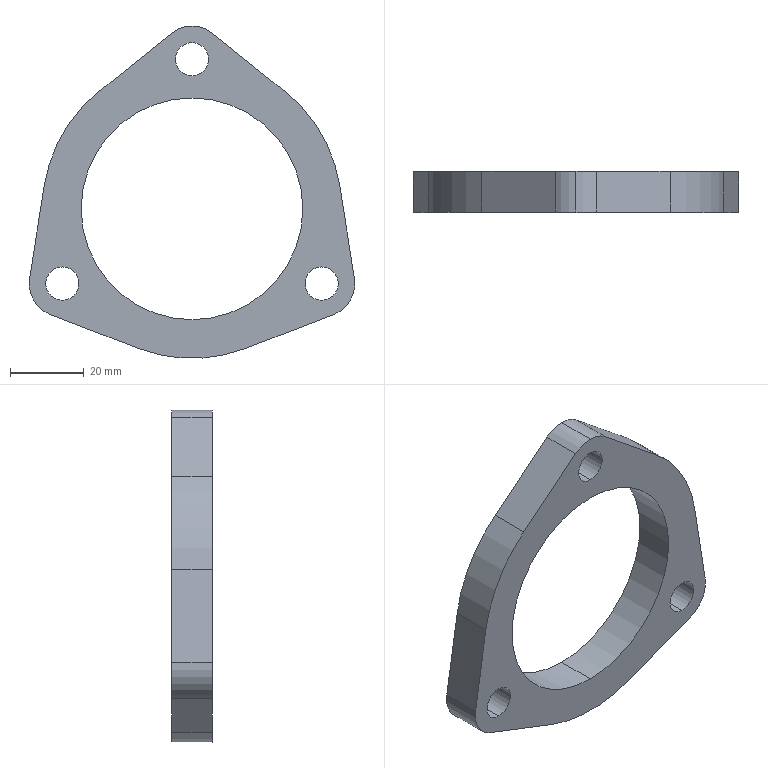Part | SolidWorks | features BaseBody 1 | 1 solid | 23 faces | box 88.148 x 11 x 90 mm | volume 30091 mm3 | cylinder 15 | plane 8 | commonest cylinder face diameters 9 x6 18 x4 81 x3 60 x2
STEP:
#1=CARTESIAN_POINT('',(0.,-60.,-30.));
#2=VERTEX_POINT('',#1);
#3=CARTESIAN_POINT('',(0.,-60.,30.));
#4=VERTEX_POINT('',#3);
#5=CARTESIAN_POINT('',(0.,-60.,0.));
#6=DIRECTION('',(0.,1.,0.));
#7=DIRECTION('',(0.,0.,1.));
#8=AXIS2_PLACEMENT_3D('',#5,#6,#7);
#9=CIRCLE('',#8,30.);
#10=EDGE_CURVE('',#2,#4,#9,.T.);
#11=ORIENTED_EDGE('',*,*,#10,.F.);
#12=CARTESIAN_POINT('',(0.,-49.,-30.));
#13=VERTEX_POINT('',#12);
#14=CARTESIAN_POINT('',(0.,-60.,-30.));
#15=DIRECTION('',(0.,1.,0.));
#16=VECTOR('',#15,1000.);
#17=LINE('',#14,#16);
#18=EDGE_CURVE('',#2,#13,#17,.T.);
#19=ORIENTED_EDGE('',*,*,#18,.T.);
#20=CARTESIAN_POINT('',(0.,-49.,30.));
#21=VERTEX_POINT('',#20);
#22=CARTESIAN_POINT('',(0.,-49.,0.));
#23=DIRECTION('',(0.,-1.,0.));
#24=DIRECTION('',(0.,0.,1.));
#25=AXIS2_PLACEMENT_3D('',#22,#23,#24);
#26=CIRCLE('',#25,30.);
#27=EDGE_CURVE('',#21,#13,#26,.T.);
#28=ORIENTED_EDGE('',*,*,#27,.F.);
#29=CARTESIAN_POINT('',(0.,-60.,30.));
#30=DIRECTION('',(0.,1.,0.));
#31=VECTOR('',#30,1000.);
#32=LINE('',#29,#31);
#33=EDGE_CURVE('',#4,#21,#32,.T.);
#34=ORIENTED_EDGE('',*,*,#33,.F.);
#35=EDGE_LOOP('',(#11,#19,#28,#34));
#36=FACE_OUTER_BOUND('',#35,.T.);
#37=CARTESIAN_POINT('',(0.,-60.,0.));
#38=DIRECTION('',(0.,1.,0.));
#39=DIRECTION('',(0.,0.,1.));
#40=AXIS2_PLACEMENT_3D('',#37,#38,#39);
#41=CYLINDRICAL_SURFACE('',#40,30.);
#42=ADVANCED_FACE('',(#36),#41,.F.);
#43=CARTESIAN_POINT('',(0.,-60.,36.));
#44=VERTEX_POINT('',#43);
#45=CARTESIAN_POINT('',(0.,-60.,45.));
#46=VERTEX_POINT('',#45);
#47=CARTESIAN_POINT('',(0.,-60.,40.5));
#48=DIRECTION('',(0.,1.,0.));
#49=DIRECTION('',(0.,0.,1.));
#50=AXIS2_PLACEMENT_3D('',#47,#48,#49);
#51=CIRCLE('',#50,4.5);
#52=EDGE_CURVE('',#44,#46,#51,.T.);
#53=ORIENTED_EDGE('',*,*,#52,.F.);
#54=CARTESIAN_POINT('',(0.,-49.,36.));
#55=VERTEX_POINT('',#54);
#56=CARTESIAN_POINT('',(0.,-60.,36.));
#57=DIRECTION('',(0.,1.,0.));
#58=VECTOR('',#57,1000.);
#59=LINE('',#56,#58);
#60=EDGE_CURVE('',#44,#55,#59,.T.);
#61=ORIENTED_EDGE('',*,*,#60,.T.);
#62=CARTESIAN_POINT('',(0.,-49.,45.));
#63=VERTEX_POINT('',#62);
#64=CARTESIAN_POINT('',(0.,-49.,40.5));
#65=DIRECTION('',(0.,-1.,0.));
#66=DIRECTION('',(0.,0.,1.));
#67=AXIS2_PLACEMENT_3D('',#64,#65,#66);
#68=CIRCLE('',#67,4.5);
#69=EDGE_CURVE('',#63,#55,#68,.T.);
#70=ORIENTED_EDGE('',*,*,#69,.F.);
#71=CARTESIAN_POINT('',(0.,-60.,45.));
#72=DIRECTION('',(0.,1.,0.));
#73=VECTOR('',#72,1000.);
#74=LINE('',#71,#73);
#75=EDGE_CURVE('',#46,#63,#74,.T.);
#76=ORIENTED_EDGE('',*,*,#75,.F.);
#77=EDGE_LOOP('',(#53,#61,#70,#76));
#78=FACE_OUTER_BOUND('',#77,.T.);
#79=CARTESIAN_POINT('',(0.,-60.,40.5));
#80=DIRECTION('',(0.,1.,0.));
#81=DIRECTION('',(0.,0.,1.));
#82=AXIS2_PLACEMENT_3D('',#79,#80,#81);
#83=CYLINDRICAL_SURFACE('',#82,4.5);
#84=ADVANCED_FACE('',(#78),#83,.F.);
#85=CARTESIAN_POINT('',(-35.074,-60.,-24.75));
#86=VERTEX_POINT('',#85);
#87=CARTESIAN_POINT('',(-35.074,-60.,-15.75));
#88=VERTEX_POINT('',#87);
#89=CARTESIAN_POINT('',(-35.074,-60.,-20.25));
#90=DIRECTION('',(0.,1.,0.));
#91=DIRECTION('',(0.,0.,1.));
#92=AXIS2_PLACEMENT_3D('',#89,#90,#91);
#93=CIRCLE('',#92,4.5);
#94=EDGE_CURVE('',#86,#88,#93,.T.);
#95=ORIENTED_EDGE('',*,*,#94,.F.);
#96=CARTESIAN_POINT('',(-35.074,-49.,-24.75));
#97=VERTEX_POINT('',#96);
#98=CARTESIAN_POINT('',(-35.074,-60.,-24.75));
#99=DIRECTION('',(0.,1.,0.));
#100=VECTOR('',#99,1000.);
#101=LINE('',#98,#100);
#102=EDGE_CURVE('',#86,#97,#101,.T.);
#103=ORIENTED_EDGE('',*,*,#102,.T.);
#104=CARTESIAN_POINT('',(-35.074,-49.,-15.75));
#105=VERTEX_POINT('',#104);
#106=CARTESIAN_POINT('',(-35.074,-49.,-20.25));
#107=DIRECTION('',(0.,-1.,0.));
#108=DIRECTION('',(0.,0.,1.));
#109=AXIS2_PLACEMENT_3D('',#106,#107,#108);
#110=CIRCLE('',#109,4.5);
#111=EDGE_CURVE('',#105,#97,#110,.T.);
#112=ORIENTED_EDGE('',*,*,#111,.F.);
#113=CARTESIAN_POINT('',(-35.074,-60.,-15.75));
#114=DIRECTION('',(0.,1.,0.));
#115=VECTOR('',#114,1000.);
#116=LINE('',#113,#115);
#117=EDGE_CURVE('',#88,#105,#116,.T.);
#118=ORIENTED_EDGE('',*,*,#117,.F.);
#119=EDGE_LOOP('',(#95,#103,#112,#118));
#120=FACE_OUTER_BOUND('',#119,.T.);
#121=CARTESIAN_POINT('',(-35.074,-60.,-20.25));
#122=DIRECTION('',(0.,1.,0.));
#123=DIRECTION('',(0.,0.,1.));
#124=AXIS2_PLACEMENT_3D('',#121,#122,#123);
#125=CYLINDRICAL_SURFACE('',#124,4.5);
#126=ADVANCED_FACE('',(#120),#125,.F.);
#127=CARTESIAN_POINT('',(35.074,-60.,-24.75));
#128=VERTEX_POINT('',#127);
#129=CARTESIAN_POINT('',(35.074,-60.,-15.75));
#130=VERTEX_POINT('',#129);
#131=CARTESIAN_POINT('',(35.074,-60.,-20.25));
#132=DIRECTION('',(0.,1.,0.));
#133=DIRECTION('',(0.,0.,1.));
#134=AXIS2_PLACEMENT_3D('',#131,#132,#133);
#135=CIRCLE('',#134,4.5);
#136=EDGE_CURVE('',#128,#130,#135,.T.);
#137=ORIENTED_EDGE('',*,*,#136,.F.);
#138=CARTESIAN_POINT('',(35.074,-49.,-24.75));
#139=VERTEX_POINT('',#138);
#140=CARTESIAN_POINT('',(35.074,-60.,-24.75));
#141=DIRECTION('',(0.,1.,0.));
#142=VECTOR('',#141,1000.);
#143=LINE('',#140,#142);
#144=EDGE_CURVE('',#128,#139,#143,.T.);
#145=ORIENTED_EDGE('',*,*,#144,.T.);
#146=CARTESIAN_POINT('',(35.074,-49.,-15.75));
#147=VERTEX_POINT('',#146);
#148=CARTESIAN_POINT('',(35.074,-49.,-20.25));
#149=DIRECTION('',(0.,-1.,0.));
#150=DIRECTION('',(0.,0.,1.));
#151=AXIS2_PLACEMENT_3D('',#148,#149,#150);
#152=CIRCLE('',#151,4.5);
#153=EDGE_CURVE('',#147,#139,#152,.T.);
#154=ORIENTED_EDGE('',*,*,#153,.F.);
#155=CARTESIAN_POINT('',(35.074,-60.,-15.75));
#156=DIRECTION('',(0.,1.,0.));
#157=VECTOR('',#156,1000.);
#158=LINE('',#155,#157);
#159=EDGE_CURVE('',#130,#147,#158,.T.);
#160=ORIENTED_EDGE('',*,*,#159,.F.);
#161=EDGE_LOOP('',(#137,#145,#154,#160));
#162=FACE_OUTER_BOUND('',#161,.T.);
#163=CARTESIAN_POINT('',(35.074,-60.,-20.25));
#164=DIRECTION('',(0.,1.,0.));
#165=DIRECTION('',(0.,0.,1.));
#166=AXIS2_PLACEMENT_3D('',#163,#164,#165);
#167=CYLINDRICAL_SURFACE('',#166,4.5);
#168=ADVANCED_FACE('',(#162),#167,.F.);
#169=CARTESIAN_POINT('',(-5.657,-60.,47.5));
#170=VERTEX_POINT('',#169);
#171=CARTESIAN_POINT('',(0.,-60.,49.5));
#172=VERTEX_POINT('',#171);
#173=CARTESIAN_POINT('',(0.,-60.,40.5));
#174=DIRECTION('',(0.,1.,0.));
#175=DIRECTION('',(0.,0.,1.));
#176=AXIS2_PLACEMENT_3D('',#173,#174,#175);
#177=CIRCLE('',#176,9.);
#178=EDGE_CURVE('',#170,#172,#177,.T.);
#179=ORIENTED_EDGE('',*,*,#178,.T.);
#180=CARTESIAN_POINT('',(0.,-49.,49.5));
#181=VERTEX_POINT('',#180);
#182=CARTESIAN_POINT('',(0.,-60.,49.5));
#183=DIRECTION('',(0.,1.,0.));
#184=VECTOR('',#183,1000.);
#185=LINE('',#182,#184);
#186=EDGE_CURVE('',#172,#181,#185,.T.);
#187=ORIENTED_EDGE('',*,*,#186,.T.);
#188=CARTESIAN_POINT('',(-5.657,-49.,47.5));
#189=VERTEX_POINT('',#188);
#190=CARTESIAN_POINT('',(0.,-49.,40.5));
#191=DIRECTION('',(0.,1.,0.));
#192=DIRECTION('',(0.,0.,1.));
#193=AXIS2_PLACEMENT_3D('',#190,#191,#192);
#194=CIRCLE('',#193,9.);
#195=EDGE_CURVE('',#189,#181,#194,.T.);
#196=ORIENTED_EDGE('',*,*,#195,.F.);
#197=CARTESIAN_POINT('',(-5.657,-60.,47.5));
#198=DIRECTION('',(0.,-1.,0.));
#199=VECTOR('',#198,1000.);
#200=LINE('',#197,#199);
#201=EDGE_CURVE('',#189,#170,#200,.T.);
#202=ORIENTED_EDGE('',*,*,#201,.T.);
#203=EDGE_LOOP('',(#179,#187,#196,#202));
#204=FACE_OUTER_BOUND('',#203,.T.);
#205=CARTESIAN_POINT('',(0.,-60.,40.5));
#206=DIRECTION('',(0.,1.,0.));
#207=DIRECTION('',(0.,0.,1.));
#208=AXIS2_PLACEMENT_3D('',#205,#206,#207);
#209=CYLINDRICAL_SURFACE('',#208,9.);
#210=ADVANCED_FACE('',(#204),#209,.T.);
#211=ORIENTED_EDGE('',*,*,#27,.T.);
#212=CARTESIAN_POINT('',(0.,-49.,0.));
#213=DIRECTION('',(0.,-1.,0.));
#214=DIRECTION('',(0.,0.,1.));
#215=AXIS2_PLACEMENT_3D('',#212,#213,#214);
#216=CIRCLE('',#215,30.);
#217=EDGE_CURVE('',#13,#21,#216,.T.);
#218=ORIENTED_EDGE('',*,*,#217,.T.);
#219=EDGE_LOOP('',(#211,#218));
#220=FACE_BOUND('',#219,.T.);
#221=ORIENTED_EDGE('',*,*,#69,.T.);
#222=CARTESIAN_POINT('',(0.,-49.,40.5));
#223=DIRECTION('',(0.,-1.,0.));
#224=DIRECTION('',(0.,0.,1.));
#225=AXIS2_PLACEMENT_3D('',#222,#223,#224);
#226=CIRCLE('',#225,4.5);
#227=EDGE_CURVE('',#55,#63,#226,.T.);
#228=ORIENTED_EDGE('',*,*,#227,.T.);
#229=EDGE_LOOP('',(#221,#228));
#230=FACE_BOUND('',#229,.T.);
#231=ORIENTED_EDGE('',*,*,#111,.T.);
#232=CARTESIAN_POINT('',(-35.074,-49.,-20.25));
#233=DIRECTION('',(0.,-1.,0.));
#234=DIRECTION('',(0.,0.,1.));
#235=AXIS2_PLACEMENT_3D('',#232,#233,#234);
#236=CIRCLE('',#235,4.5);
#237=EDGE_CURVE('',#97,#105,#236,.T.);
#238=ORIENTED_EDGE('',*,*,#237,.T.);
#239=EDGE_LOOP('',(#231,#238));
#240=FACE_BOUND('',#239,.T.);
#241=ORIENTED_EDGE('',*,*,#153,.T.);
#242=CARTESIAN_POINT('',(35.074,-49.,-20.25));
#243=DIRECTION('',(0.,-1.,0.));
#244=DIRECTION('',(0.,0.,1.));
#245=AXIS2_PLACEMENT_3D('',#242,#243,#244);
#246=CIRCLE('',#245,4.5);
#247=EDGE_CURVE('',#139,#147,#246,.T.);
#248=ORIENTED_EDGE('',*,*,#247,.T.);
#249=EDGE_LOOP('',(#241,#248));
#250=FACE_BOUND('',#249,.T.);
#251=CARTESIAN_POINT('',(38.308,-49.,-28.649));
#252=VERTEX_POINT('',#251);
#253=CARTESIAN_POINT('',(14.552,-49.,-37.795));
#254=VERTEX_POINT('',#253);
#255=CARTESIAN_POINT('',(38.308,-49.,-28.649));
#256=DIRECTION('',(-0.9332,0.,-0.3593));
#257=VECTOR('',#256,1000.);
#258=LINE('',#255,#257);
#259=EDGE_CURVE('',#252,#254,#258,.T.);
#260=ORIENTED_EDGE('',*,*,#259,.T.);
#261=CARTESIAN_POINT('',(-14.552,-49.,-37.795));
#262=VERTEX_POINT('',#261);
#263=CARTESIAN_POINT('',(0.,-49.,0.));
#264=DIRECTION('',(0.,1.,0.));
#265=DIRECTION('',(0.,0.,1.));
#266=AXIS2_PLACEMENT_3D('',#263,#264,#265);
#267=CIRCLE('',#266,40.5);
#268=EDGE_CURVE('',#254,#262,#267,.T.);
#269=ORIENTED_EDGE('',*,*,#268,.T.);
#270=CARTESIAN_POINT('',(-38.308,-49.,-28.649));
#271=VERTEX_POINT('',#270);
#272=CARTESIAN_POINT('',(-14.552,-49.,-37.795));
#273=DIRECTION('',(-0.9332,0.,0.3593));
#274=VECTOR('',#273,1000.);
#275=LINE('',#272,#274);
#276=EDGE_CURVE('',#262,#271,#275,.T.);
#277=ORIENTED_EDGE('',*,*,#276,.T.);
#278=CARTESIAN_POINT('',(-43.965,-49.,-18.851));
#279=VERTEX_POINT('',#278);
#280=CARTESIAN_POINT('',(-35.074,-49.,-20.25));
#281=DIRECTION('',(0.,1.,0.));
#282=DIRECTION('',(0.,0.,1.));
#283=AXIS2_PLACEMENT_3D('',#280,#281,#282);
#284=CIRCLE('',#283,9.);
#285=EDGE_CURVE('',#271,#279,#284,.T.);
#286=ORIENTED_EDGE('',*,*,#285,.T.);
#287=CARTESIAN_POINT('',(-40.008,-49.,6.295));
#288=VERTEX_POINT('',#287);
#289=CARTESIAN_POINT('',(-43.965,-49.,-18.851));
#290=DIRECTION('',(0.1554,0.,0.9878));
#291=VECTOR('',#290,1000.);
#292=LINE('',#289,#291);
#293=EDGE_CURVE('',#279,#288,#292,.T.);
#294=ORIENTED_EDGE('',*,*,#293,.T.);
#295=CARTESIAN_POINT('',(-25.456,-49.,31.5));
#296=VERTEX_POINT('',#295);
#297=CARTESIAN_POINT('',(0.,-49.,0.));
#298=DIRECTION('',(0.,1.,0.));
#299=DIRECTION('',(0.,0.,1.));
#300=AXIS2_PLACEMENT_3D('',#297,#298,#299);
#301=CIRCLE('',#300,40.5);
#302=EDGE_CURVE('',#288,#296,#301,.T.);
#303=ORIENTED_EDGE('',*,*,#302,.T.);
#304=CARTESIAN_POINT('',(-25.456,-49.,31.5));
#305=DIRECTION('',(0.7778,0.,0.6285));
#306=VECTOR('',#305,1000.);
#307=LINE('',#304,#306);
#308=EDGE_CURVE('',#296,#189,#307,.T.);
#309=ORIENTED_EDGE('',*,*,#308,.T.);
#310=ORIENTED_EDGE('',*,*,#195,.T.);
#311=CARTESIAN_POINT('',(5.657,-49.,47.5));
#312=VERTEX_POINT('',#311);
#313=CARTESIAN_POINT('',(0.,-49.,40.5));
#314=DIRECTION('',(0.,1.,0.));
#315=DIRECTION('',(0.,0.,1.));
#316=AXIS2_PLACEMENT_3D('',#313,#314,#315);
#317=CIRCLE('',#316,9.);
#318=EDGE_CURVE('',#181,#312,#317,.T.);
#319=ORIENTED_EDGE('',*,*,#318,.T.);
#320=CARTESIAN_POINT('',(25.456,-49.,31.5));
#321=VERTEX_POINT('',#320);
#322=CARTESIAN_POINT('',(5.657,-49.,47.5));
#323=DIRECTION('',(0.7778,0.,-0.6285));
#324=VECTOR('',#323,1000.);
#325=LINE('',#322,#324);
#326=EDGE_CURVE('',#312,#321,#325,.T.);
#327=ORIENTED_EDGE('',*,*,#326,.T.);
#328=CARTESIAN_POINT('',(40.008,-49.,6.295));
#329=VERTEX_POINT('',#328);
#330=CARTESIAN_POINT('',(0.,-49.,0.));
#331=DIRECTION('',(0.,1.,0.));
#332=DIRECTION('',(0.,0.,1.));
#333=AXIS2_PLACEMENT_3D('',#330,#331,#332);
#334=CIRCLE('',#333,40.5);
#335=EDGE_CURVE('',#321,#329,#334,.T.);
#336=ORIENTED_EDGE('',*,*,#335,.T.);
#337=CARTESIAN_POINT('',(43.965,-49.,-18.851));
#338=VERTEX_POINT('',#337);
#339=CARTESIAN_POINT('',(40.008,-49.,6.295));
#340=DIRECTION('',(0.1554,0.,-0.9878));
#341=VECTOR('',#340,1000.);
#342=LINE('',#339,#341);
#343=EDGE_CURVE('',#329,#338,#342,.T.);
#344=ORIENTED_EDGE('',*,*,#343,.T.);
#345=CARTESIAN_POINT('',(35.074,-49.,-20.25));
#346=DIRECTION('',(0.,1.,0.));
#347=DIRECTION('',(0.,0.,1.));
#348=AXIS2_PLACEMENT_3D('',#345,#346,#347);
#349=CIRCLE('',#348,9.);
#350=EDGE_CURVE('',#338,#252,#349,.T.);
#351=ORIENTED_EDGE('',*,*,#350,.T.);
#352=EDGE_LOOP('',(#260,#269,#277,#286,#294,#303,#309,#310,#319,#327,#336,#344,#351));
#353=FACE_OUTER_BOUND('',#352,.T.);
#354=CARTESIAN_POINT('',(0.0009407,-49.,4.506));
#355=DIRECTION('',(0.,1.,0.));
#356=DIRECTION('',(0.,0.,1.));
#357=AXIS2_PLACEMENT_3D('',#354,#355,#356);
#358=PLANE('',#357);
#359=ADVANCED_FACE('',(#220,#230,#240,#250,#353),#358,.T.);
#360=ORIENTED_EDGE('',*,*,#18,.F.);
#361=CARTESIAN_POINT('',(0.,-60.,0.));
#362=DIRECTION('',(0.,1.,0.));
#363=DIRECTION('',(0.,0.,1.));
#364=AXIS2_PLACEMENT_3D('',#361,#362,#363);
#365=CIRCLE('',#364,30.);
#366=EDGE_CURVE('',#4,#2,#365,.T.);
#367=ORIENTED_EDGE('',*,*,#366,.F.);
#368=ORIENTED_EDGE('',*,*,#33,.T.);
#369=ORIENTED_EDGE('',*,*,#217,.F.);
#370=EDGE_LOOP('',(#360,#367,#368,#369));
#371=FACE_OUTER_BOUND('',#370,.T.);
#372=CARTESIAN_POINT('',(0.,-60.,0.));
#373=DIRECTION('',(0.,1.,0.));
#374=DIRECTION('',(0.,0.,1.));
#375=AXIS2_PLACEMENT_3D('',#372,#373,#374);
#376=CYLINDRICAL_SURFACE('',#375,30.);
#377=ADVANCED_FACE('',(#371),#376,.F.);
#378=ORIENTED_EDGE('',*,*,#60,.F.);
#379=CARTESIAN_POINT('',(0.,-60.,40.5));
#380=DIRECTION('',(0.,1.,0.));
#381=DIRECTION('',(0.,0.,1.));
#382=AXIS2_PLACEMENT_3D('',#379,#380,#381);
#383=CIRCLE('',#382,4.5);
#384=EDGE_CURVE('',#46,#44,#383,.T.);
#385=ORIENTED_EDGE('',*,*,#384,.F.);
#386=ORIENTED_EDGE('',*,*,#75,.T.);
#387=ORIENTED_EDGE('',*,*,#227,.F.);
#388=EDGE_LOOP('',(#378,#385,#386,#387));
#389=FACE_OUTER_BOUND('',#388,.T.);
#390=CARTESIAN_POINT('',(0.,-60.,40.5));
#391=DIRECTION('',(0.,1.,0.));
#392=DIRECTION('',(0.,0.,1.));
#393=AXIS2_PLACEMENT_3D('',#390,#391,#392);
#394=CYLINDRICAL_SURFACE('',#393,4.5);
#395=ADVANCED_FACE('',(#389),#394,.F.);
#396=ORIENTED_EDGE('',*,*,#102,.F.);
#397=CARTESIAN_POINT('',(-35.074,-60.,-20.25));
#398=DIRECTION('',(0.,1.,0.));
#399=DIRECTION('',(0.,0.,1.));
#400=AXIS2_PLACEMENT_3D('',#397,#398,#399);
#401=CIRCLE('',#400,4.5);
#402=EDGE_CURVE('',#88,#86,#401,.T.);
#403=ORIENTED_EDGE('',*,*,#402,.F.);
#404=ORIENTED_EDGE('',*,*,#117,.T.);
#405=ORIENTED_EDGE('',*,*,#237,.F.);
#406=EDGE_LOOP('',(#396,#403,#404,#405));
#407=FACE_OUTER_BOUND('',#406,.T.);
#408=CARTESIAN_POINT('',(-35.074,-60.,-20.25));
#409=DIRECTION('',(0.,1.,0.));
#410=DIRECTION('',(0.,0.,1.));
#411=AXIS2_PLACEMENT_3D('',#408,#409,#410);
#412=CYLINDRICAL_SURFACE('',#411,4.5);
#413=ADVANCED_FACE('',(#407),#412,.F.);
#414=ORIENTED_EDGE('',*,*,#144,.F.);
#415=CARTESIAN_POINT('',(35.074,-60.,-20.25));
#416=DIRECTION('',(0.,1.,0.));
#417=DIRECTION('',(0.,0.,1.));
#418=AXIS2_PLACEMENT_3D('',#415,#416,#417);
#419=CIRCLE('',#418,4.5);
#420=EDGE_CURVE('',#130,#128,#419,.T.);
#421=ORIENTED_EDGE('',*,*,#420,.F.);
#422=ORIENTED_EDGE('',*,*,#159,.T.);
#423=ORIENTED_EDGE('',*,*,#247,.F.);
#424=EDGE_LOOP('',(#414,#421,#422,#423));
#425=FACE_OUTER_BOUND('',#424,.T.);
#426=CARTESIAN_POINT('',(35.074,-60.,-20.25));
#427=DIRECTION('',(0.,1.,0.));
#428=DIRECTION('',(0.,0.,1.));
#429=AXIS2_PLACEMENT_3D('',#426,#427,#428);
#430=CYLINDRICAL_SURFACE('',#429,4.5);
#431=ADVANCED_FACE('',(#425),#430,.F.);
#432=CARTESIAN_POINT('',(14.552,-60.,-37.795));
#433=VERTEX_POINT('',#432);
#434=CARTESIAN_POINT('',(14.552,-60.,-37.795));
#435=DIRECTION('',(0.,-1.,0.));
#436=VECTOR('',#435,1000.);
#437=LINE('',#434,#436);
#438=EDGE_CURVE('',#254,#433,#437,.T.);
#439=ORIENTED_EDGE('',*,*,#438,.T.);
#440=CARTESIAN_POINT('',(-14.552,-60.,-37.795));
#441=VERTEX_POINT('',#440);
#442=CARTESIAN_POINT('',(0.,-60.,0.));
#443=DIRECTION('',(0.,1.,0.));
#444=DIRECTION('',(0.,0.,1.));
#445=AXIS2_PLACEMENT_3D('',#442,#443,#444);
#446=CIRCLE('',#445,40.5);
#447=EDGE_CURVE('',#433,#441,#446,.T.);
#448=ORIENTED_EDGE('',*,*,#447,.T.);
#449=CARTESIAN_POINT('',(-14.552,-60.,-37.795));
#450=DIRECTION('',(0.,1.,0.));
#451=VECTOR('',#450,1000.);
#452=LINE('',#449,#451);
#453=EDGE_CURVE('',#441,#262,#452,.T.);
#454=ORIENTED_EDGE('',*,*,#453,.T.);
#455=ORIENTED_EDGE('',*,*,#268,.F.);
#456=EDGE_LOOP('',(#439,#448,#454,#455));
#457=FACE_OUTER_BOUND('',#456,.T.);
#458=CARTESIAN_POINT('',(0.,-60.,0.));
#459=DIRECTION('',(0.,1.,0.));
#460=DIRECTION('',(0.,0.,1.));
#461=AXIS2_PLACEMENT_3D('',#458,#459,#460);
#462=CYLINDRICAL_SURFACE('',#461,40.5);
#463=ADVANCED_FACE('',(#457),#462,.T.);
#464=CARTESIAN_POINT('',(38.308,-60.,-28.649));
#465=VERTEX_POINT('',#464);
#466=CARTESIAN_POINT('',(38.308,-54.5,-28.649));
#467=DIRECTION('',(0.,1.,0.));
#468=VECTOR('',#467,1000.);
#469=LINE('',#466,#468);
#470=EDGE_CURVE('',#465,#252,#469,.T.);
#471=ORIENTED_EDGE('',*,*,#470,.F.);
#472=CARTESIAN_POINT('',(26.43,-60.,-33.222));
#473=DIRECTION('',(0.9332,0.,0.3593));
#474=VECTOR('',#473,1000.);
#475=LINE('',#472,#474);
#476=EDGE_CURVE('',#433,#465,#475,.T.);
#477=ORIENTED_EDGE('',*,*,#476,.F.);
#478=ORIENTED_EDGE('',*,*,#438,.F.);
#479=ORIENTED_EDGE('',*,*,#259,.F.);
#480=EDGE_LOOP('',(#471,#477,#478,#479));
#481=FACE_OUTER_BOUND('',#480,.T.);
#482=CARTESIAN_POINT('',(26.43,-54.5,-33.222));
#483=DIRECTION('',(-0.3593,0.,0.9332));
#484=DIRECTION('',(0.9332,0.,0.3593));
#485=AXIS2_PLACEMENT_3D('',#482,#483,#484);
#486=PLANE('',#485);
#487=ADVANCED_FACE('',(#481),#486,.F.);
#488=CARTESIAN_POINT('',(43.965,-60.,-18.851));
#489=VERTEX_POINT('',#488);
#490=CARTESIAN_POINT('',(35.074,-60.,-20.25));
#491=DIRECTION('',(0.,1.,0.));
#492=DIRECTION('',(0.,0.,1.));
#493=AXIS2_PLACEMENT_3D('',#490,#491,#492);
#494=CIRCLE('',#493,9.);
#495=EDGE_CURVE('',#489,#465,#494,.T.);
#496=ORIENTED_EDGE('',*,*,#495,.T.);
#497=ORIENTED_EDGE('',*,*,#470,.T.);
#498=ORIENTED_EDGE('',*,*,#350,.F.);
#499=CARTESIAN_POINT('',(43.965,-60.,-18.851));
#500=DIRECTION('',(0.,-1.,0.));
#501=VECTOR('',#500,1000.);
#502=LINE('',#499,#501);
#503=EDGE_CURVE('',#338,#489,#502,.T.);
#504=ORIENTED_EDGE('',*,*,#503,.T.);
#505=EDGE_LOOP('',(#496,#497,#498,#504));
#506=FACE_OUTER_BOUND('',#505,.T.);
#507=CARTESIAN_POINT('',(35.074,-60.,-20.25));
#508=DIRECTION('',(0.,1.,0.));
#509=DIRECTION('',(0.,0.,1.));
#510=AXIS2_PLACEMENT_3D('',#507,#508,#509);
#511=CYLINDRICAL_SURFACE('',#510,9.);
#512=ADVANCED_FACE('',(#506),#511,.T.);
#513=CARTESIAN_POINT('',(40.008,-60.,6.295));
#514=VERTEX_POINT('',#513);
#515=CARTESIAN_POINT('',(41.986,-60.,-6.278));
#516=DIRECTION('',(0.1554,0.,-0.9878));
#517=VECTOR('',#516,1000.);
#518=LINE('',#515,#517);
#519=EDGE_CURVE('',#514,#489,#518,.T.);
#520=ORIENTED_EDGE('',*,*,#519,.T.);
#521=ORIENTED_EDGE('',*,*,#503,.F.);
#522=ORIENTED_EDGE('',*,*,#343,.F.);
#523=CARTESIAN_POINT('',(40.008,-54.5,6.295));
#524=DIRECTION('',(0.,-1.,0.));
#525=VECTOR('',#524,1000.);
#526=LINE('',#523,#525);
#527=EDGE_CURVE('',#329,#514,#526,.T.);
#528=ORIENTED_EDGE('',*,*,#527,.T.);
#529=EDGE_LOOP('',(#520,#521,#522,#528));
#530=FACE_OUTER_BOUND('',#529,.T.);
#531=CARTESIAN_POINT('',(41.986,-54.5,-6.278));
#532=DIRECTION('',(0.9878,0.,0.1554));
#533=DIRECTION('',(0.1554,0.,-0.9878));
#534=AXIS2_PLACEMENT_3D('',#531,#532,#533);
#535=PLANE('',#534);
#536=ADVANCED_FACE('',(#530),#535,.T.);
#537=CARTESIAN_POINT('',(25.456,-60.,31.5));
#538=VERTEX_POINT('',#537);
#539=CARTESIAN_POINT('',(25.456,-60.,31.5));
#540=DIRECTION('',(0.,-1.,0.));
#541=VECTOR('',#540,1000.);
#542=LINE('',#539,#541);
#543=EDGE_CURVE('',#321,#538,#542,.T.);
#544=ORIENTED_EDGE('',*,*,#543,.T.);
#545=CARTESIAN_POINT('',(0.,-60.,0.));
#546=DIRECTION('',(0.,1.,0.));
#547=DIRECTION('',(0.,0.,1.));
#548=AXIS2_PLACEMENT_3D('',#545,#546,#547);
#549=CIRCLE('',#548,40.5);
#550=EDGE_CURVE('',#538,#514,#549,.T.);
#551=ORIENTED_EDGE('',*,*,#550,.T.);
#552=ORIENTED_EDGE('',*,*,#527,.F.);
#553=ORIENTED_EDGE('',*,*,#335,.F.);
#554=EDGE_LOOP('',(#544,#551,#552,#553));
#555=FACE_OUTER_BOUND('',#554,.T.);
#556=CARTESIAN_POINT('',(0.,-60.,0.));
#557=DIRECTION('',(0.,1.,0.));
#558=DIRECTION('',(0.,0.,1.));
#559=AXIS2_PLACEMENT_3D('',#556,#557,#558);
#560=CYLINDRICAL_SURFACE('',#559,40.5);
#561=ADVANCED_FACE('',(#555),#560,.T.);
#562=CARTESIAN_POINT('',(5.657,-60.,47.5));
#563=VERTEX_POINT('',#562);
#564=CARTESIAN_POINT('',(15.556,-60.,39.5));
#565=DIRECTION('',(0.7778,0.,-0.6285));
#566=VECTOR('',#565,1000.);
#567=LINE('',#564,#566);
#568=EDGE_CURVE('',#563,#538,#567,.T.);
#569=ORIENTED_EDGE('',*,*,#568,.T.);
#570=ORIENTED_EDGE('',*,*,#543,.F.);
#571=ORIENTED_EDGE('',*,*,#326,.F.);
#572=CARTESIAN_POINT('',(5.657,-54.5,47.5));
#573=DIRECTION('',(0.,-1.,0.));
#574=VECTOR('',#573,1000.);
#575=LINE('',#572,#574);
#576=EDGE_CURVE('',#312,#563,#575,.T.);
#577=ORIENTED_EDGE('',*,*,#576,.T.);
#578=EDGE_LOOP('',(#569,#570,#571,#577));
#579=FACE_OUTER_BOUND('',#578,.T.);
#580=CARTESIAN_POINT('',(15.556,-54.5,39.5));
#581=DIRECTION('',(0.6285,0.,0.7778));
#582=DIRECTION('',(0.7778,0.,-0.6285));
#583=AXIS2_PLACEMENT_3D('',#580,#581,#582);
#584=PLANE('',#583);
#585=ADVANCED_FACE('',(#579),#584,.T.);
#586=ORIENTED_EDGE('',*,*,#186,.F.);
#587=CARTESIAN_POINT('',(0.,-60.,40.5));
#588=DIRECTION('',(0.,1.,0.));
#589=DIRECTION('',(0.,0.,1.));
#590=AXIS2_PLACEMENT_3D('',#587,#588,#589);
#591=CIRCLE('',#590,9.);
#592=EDGE_CURVE('',#172,#563,#591,.T.);
#593=ORIENTED_EDGE('',*,*,#592,.T.);
#594=ORIENTED_EDGE('',*,*,#576,.F.);
#595=ORIENTED_EDGE('',*,*,#318,.F.);
#596=EDGE_LOOP('',(#586,#593,#594,#595));
#597=FACE_OUTER_BOUND('',#596,.T.);
#598=CARTESIAN_POINT('',(0.,-60.,40.5));
#599=DIRECTION('',(0.,1.,0.));
#600=DIRECTION('',(0.,0.,1.));
#601=AXIS2_PLACEMENT_3D('',#598,#599,#600);
#602=CYLINDRICAL_SURFACE('',#601,9.);
#603=ADVANCED_FACE('',(#597),#602,.T.);
#604=CARTESIAN_POINT('',(-25.456,-60.,31.5));
#605=VERTEX_POINT('',#604);
#606=CARTESIAN_POINT('',(-15.556,-60.,39.5));
#607=DIRECTION('',(0.7778,0.,0.6285));
#608=VECTOR('',#607,1000.);
#609=LINE('',#606,#608);
#610=EDGE_CURVE('',#605,#170,#609,.T.);
#611=ORIENTED_EDGE('',*,*,#610,.T.);
#612=ORIENTED_EDGE('',*,*,#201,.F.);
#613=ORIENTED_EDGE('',*,*,#308,.F.);
#614=CARTESIAN_POINT('',(-25.456,-54.5,31.5));
#615=DIRECTION('',(0.,-1.,0.));
#616=VECTOR('',#615,1000.);
#617=LINE('',#614,#616);
#618=EDGE_CURVE('',#296,#605,#617,.T.);
#619=ORIENTED_EDGE('',*,*,#618,.T.);
#620=EDGE_LOOP('',(#611,#612,#613,#619));
#621=FACE_OUTER_BOUND('',#620,.T.);
#622=CARTESIAN_POINT('',(-15.556,-54.5,39.5));
#623=DIRECTION('',(-0.6285,0.,0.7778));
#624=DIRECTION('',(0.7778,0.,0.6285));
#625=AXIS2_PLACEMENT_3D('',#622,#623,#624);
#626=PLANE('',#625);
#627=ADVANCED_FACE('',(#621),#626,.T.);
#628=CARTESIAN_POINT('',(-40.008,-60.,6.295));
#629=VERTEX_POINT('',#628);
#630=CARTESIAN_POINT('',(-40.008,-60.,6.295));
#631=DIRECTION('',(0.,-1.,0.));
#632=VECTOR('',#631,1000.);
#633=LINE('',#630,#632);
#634=EDGE_CURVE('',#288,#629,#633,.T.);
#635=ORIENTED_EDGE('',*,*,#634,.T.);
#636=CARTESIAN_POINT('',(0.,-60.,0.));
#637=DIRECTION('',(0.,1.,0.));
#638=DIRECTION('',(0.,0.,1.));
#639=AXIS2_PLACEMENT_3D('',#636,#637,#638);
#640=CIRCLE('',#639,40.5);
#641=EDGE_CURVE('',#629,#605,#640,.T.);
#642=ORIENTED_EDGE('',*,*,#641,.T.);
#643=ORIENTED_EDGE('',*,*,#618,.F.);
#644=ORIENTED_EDGE('',*,*,#302,.F.);
#645=EDGE_LOOP('',(#635,#642,#643,#644));
#646=FACE_OUTER_BOUND('',#645,.T.);
#647=CARTESIAN_POINT('',(0.,-60.,0.));
#648=DIRECTION('',(0.,1.,0.));
#649=DIRECTION('',(0.,0.,1.));
#650=AXIS2_PLACEMENT_3D('',#647,#648,#649);
#651=CYLINDRICAL_SURFACE('',#650,40.5);
#652=ADVANCED_FACE('',(#646),#651,.T.);
#653=CARTESIAN_POINT('',(-43.965,-60.,-18.851));
#654=VERTEX_POINT('',#653);
#655=CARTESIAN_POINT('',(-43.965,-54.5,-18.851));
#656=DIRECTION('',(0.,1.,0.));
#657=VECTOR('',#656,1000.);
#658=LINE('',#655,#657);
#659=EDGE_CURVE('',#654,#279,#658,.T.);
#660=ORIENTED_EDGE('',*,*,#659,.F.);
#661=CARTESIAN_POINT('',(-41.986,-60.,-6.278));
#662=DIRECTION('',(-0.1554,0.,-0.9878));
#663=VECTOR('',#662,1000.);
#664=LINE('',#661,#663);
#665=EDGE_CURVE('',#629,#654,#664,.T.);
#666=ORIENTED_EDGE('',*,*,#665,.F.);
#667=ORIENTED_EDGE('',*,*,#634,.F.);
#668=ORIENTED_EDGE('',*,*,#293,.F.);
#669=EDGE_LOOP('',(#660,#666,#667,#668));
#670=FACE_OUTER_BOUND('',#669,.T.);
#671=CARTESIAN_POINT('',(-41.986,-54.5,-6.278));
#672=DIRECTION('',(0.9878,0.,-0.1554));
#673=DIRECTION('',(-0.1554,0.,-0.9878));
#674=AXIS2_PLACEMENT_3D('',#671,#672,#673);
#675=PLANE('',#674);
#676=ADVANCED_FACE('',(#670),#675,.F.);
#677=CARTESIAN_POINT('',(-38.308,-60.,-28.649));
#678=VERTEX_POINT('',#677);
#679=CARTESIAN_POINT('',(-38.308,-60.,-28.649));
#680=DIRECTION('',(0.,-1.,0.));
#681=VECTOR('',#680,1000.);
#682=LINE('',#679,#681);
#683=EDGE_CURVE('',#271,#678,#682,.T.);
#684=ORIENTED_EDGE('',*,*,#683,.T.);
#685=CARTESIAN_POINT('',(-35.074,-60.,-20.25));
#686=DIRECTION('',(0.,1.,0.));
#687=DIRECTION('',(0.,0.,1.));
#688=AXIS2_PLACEMENT_3D('',#685,#686,#687);
#689=CIRCLE('',#688,9.);
#690=EDGE_CURVE('',#678,#654,#689,.T.);
#691=ORIENTED_EDGE('',*,*,#690,.T.);
#692=ORIENTED_EDGE('',*,*,#659,.T.);
#693=ORIENTED_EDGE('',*,*,#285,.F.);
#694=EDGE_LOOP('',(#684,#691,#692,#693));
#695=FACE_OUTER_BOUND('',#694,.T.);
#696=CARTESIAN_POINT('',(-35.074,-60.,-20.25));
#697=DIRECTION('',(0.,1.,0.));
#698=DIRECTION('',(0.,0.,1.));
#699=AXIS2_PLACEMENT_3D('',#696,#697,#698);
#700=CYLINDRICAL_SURFACE('',#699,9.);
#701=ADVANCED_FACE('',(#695),#700,.T.);
#702=ORIENTED_EDGE('',*,*,#453,.F.);
#703=CARTESIAN_POINT('',(-26.43,-60.,-33.222));
#704=DIRECTION('',(0.9332,0.,-0.3593));
#705=VECTOR('',#704,1000.);
#706=LINE('',#703,#705);
#707=EDGE_CURVE('',#678,#441,#706,.T.);
#708=ORIENTED_EDGE('',*,*,#707,.F.);
#709=ORIENTED_EDGE('',*,*,#683,.F.);
#710=ORIENTED_EDGE('',*,*,#276,.F.);
#711=EDGE_LOOP('',(#702,#708,#709,#710));
#712=FACE_OUTER_BOUND('',#711,.T.);
#713=CARTESIAN_POINT('',(-26.43,-54.5,-33.222));
#714=DIRECTION('',(0.3593,0.,0.9332));
#715=DIRECTION('',(0.9332,0.,-0.3593));
#716=AXIS2_PLACEMENT_3D('',#713,#714,#715);
#717=PLANE('',#716);
#718=ADVANCED_FACE('',(#712),#717,.F.);
#719=ORIENTED_EDGE('',*,*,#366,.T.);
#720=ORIENTED_EDGE('',*,*,#10,.T.);
#721=EDGE_LOOP('',(#719,#720));
#722=FACE_BOUND('',#721,.T.);
#723=ORIENTED_EDGE('',*,*,#384,.T.);
#724=ORIENTED_EDGE('',*,*,#52,.T.);
#725=EDGE_LOOP('',(#723,#724));
#726=FACE_BOUND('',#725,.T.);
#727=ORIENTED_EDGE('',*,*,#402,.T.);
#728=ORIENTED_EDGE('',*,*,#94,.T.);
#729=EDGE_LOOP('',(#727,#728));
#730=FACE_BOUND('',#729,.T.);
#731=ORIENTED_EDGE('',*,*,#420,.T.);
#732=ORIENTED_EDGE('',*,*,#136,.T.);
#733=EDGE_LOOP('',(#731,#732));
#734=FACE_BOUND('',#733,.T.);
#735=ORIENTED_EDGE('',*,*,#495,.F.);
#736=ORIENTED_EDGE('',*,*,#519,.F.);
#737=ORIENTED_EDGE('',*,*,#550,.F.);
#738=ORIENTED_EDGE('',*,*,#568,.F.);
#739=ORIENTED_EDGE('',*,*,#592,.F.);
#740=ORIENTED_EDGE('',*,*,#178,.F.);
#741=ORIENTED_EDGE('',*,*,#610,.F.);
#742=ORIENTED_EDGE('',*,*,#641,.F.);
#743=ORIENTED_EDGE('',*,*,#665,.T.);
#744=ORIENTED_EDGE('',*,*,#690,.F.);
#745=ORIENTED_EDGE('',*,*,#707,.T.);
#746=ORIENTED_EDGE('',*,*,#447,.F.);
#747=ORIENTED_EDGE('',*,*,#476,.T.);
#748=EDGE_LOOP('',(#735,#736,#737,#738,#739,#740,#741,#742,#743,#744,#745,#746,#747));
#749=FACE_OUTER_BOUND('',#748,.T.);
#750=CARTESIAN_POINT('',(0.0009407,-60.,4.506));
#751=DIRECTION('',(0.,1.,0.));
#752=DIRECTION('',(0.,0.,1.));
#753=AXIS2_PLACEMENT_3D('',#750,#751,#752);
#754=PLANE('',#753);
#755=ADVANCED_FACE('',(#722,#726,#730,#734,#749),#754,.F.);
#756=CLOSED_SHELL('',(#42,#84,#126,#168,#210,#359,#377,#395,#413,#431,#463,#487,#512,#536,#561,#585,#603,#627,#652,#676,#701,#718,#755));
#757=MANIFOLD_SOLID_BREP('',#756);
#758=CARTESIAN_POINT('',(0.,0.,0.));
#759=DIRECTION('',(0.,0.,1.));
#760=DIRECTION('',(1.,0.,0.));
#761=AXIS2_PLACEMENT_3D('',#758,#759,#760);
#762=(LENGTH_UNIT()NAMED_UNIT(*)SI_UNIT(.MILLI.,.METRE.));
#763=UNCERTAINTY_MEASURE_WITH_UNIT(LENGTH_MEASURE(0.00001),#762,'','');
#764=(NAMED_UNIT(*)PLANE_ANGLE_UNIT()SI_UNIT($,.RADIAN.));
#765=(NAMED_UNIT(*)SI_UNIT($,.STERADIAN.)SOLID_ANGLE_UNIT());
#766=(GEOMETRIC_REPRESENTATION_CONTEXT(3)GLOBAL_UNCERTAINTY_ASSIGNED_CONTEXT((#763))GLOBAL_UNIT_ASSIGNED_CONTEXT((#762,#764,#765))REPRESENTATION_CONTEXT('',''));
#767=ADVANCED_BREP_SHAPE_REPRESENTATION('',(#757,#761),#766);